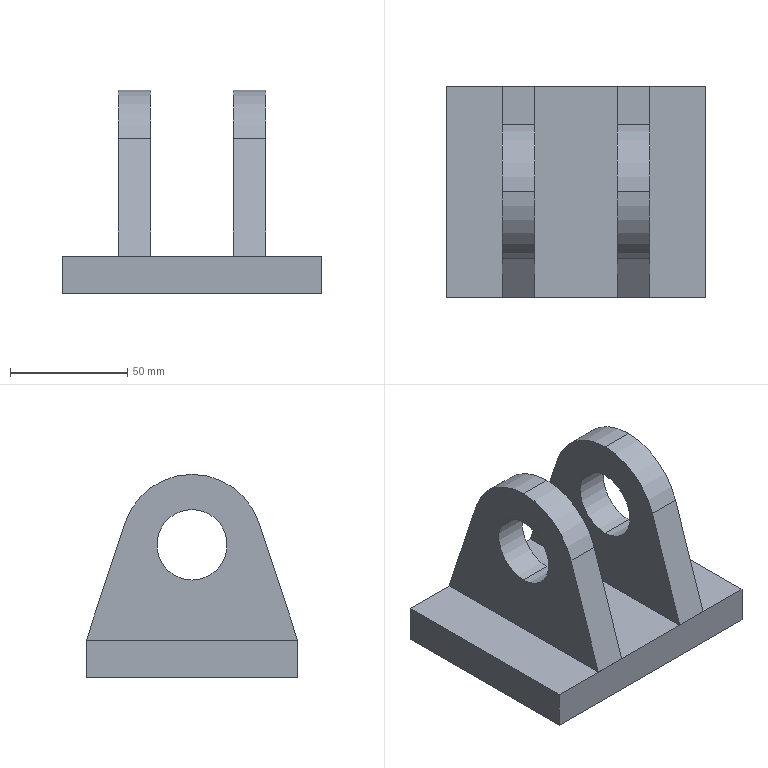Part | SolidWorks | features ICE 2, Extrusion 1, MirrorSolid 1 | 3 solids | 24 faces | box 110 x 90 x 86.592 mm | volume 265530 mm3 | plane 16 | cylinder 8 | commonest cylinder face diameters 30 x4 60 x4
STEP:
#1=CARTESIAN_POINT('',(55.,-45.,0.));
#2=VERTEX_POINT('',#1);
#3=CARTESIAN_POINT('',(55.,45.,0.));
#4=VERTEX_POINT('',#3);
#5=CARTESIAN_POINT('',(55.,-45.,0.));
#6=DIRECTION('',(0.,1.,0.));
#7=VECTOR('',#6,1000.);
#8=LINE('',#5,#7);
#9=EDGE_CURVE('',#2,#4,#8,.T.);
#10=ORIENTED_EDGE('',*,*,#9,.T.);
#11=CARTESIAN_POINT('',(55.,45.,16.));
#12=VERTEX_POINT('',#11);
#13=CARTESIAN_POINT('',(55.,45.,16.));
#14=DIRECTION('',(0.,0.,-1.));
#15=VECTOR('',#14,1000.);
#16=LINE('',#13,#15);
#17=EDGE_CURVE('',#12,#4,#16,.T.);
#18=ORIENTED_EDGE('',*,*,#17,.F.);
#19=CARTESIAN_POINT('',(55.,-45.,16.));
#20=VERTEX_POINT('',#19);
#21=CARTESIAN_POINT('',(55.,-45.,16.));
#22=DIRECTION('',(0.,1.,0.));
#23=VECTOR('',#22,1000.);
#24=LINE('',#21,#23);
#25=EDGE_CURVE('',#20,#12,#24,.T.);
#26=ORIENTED_EDGE('',*,*,#25,.F.);
#27=CARTESIAN_POINT('',(55.,-45.,16.));
#28=DIRECTION('',(0.,0.,-1.));
#29=VECTOR('',#28,1000.);
#30=LINE('',#27,#29);
#31=EDGE_CURVE('',#20,#2,#30,.T.);
#32=ORIENTED_EDGE('',*,*,#31,.T.);
#33=EDGE_LOOP('',(#10,#18,#26,#32));
#34=FACE_OUTER_BOUND('',#33,.T.);
#35=CARTESIAN_POINT('',(55.,-45.,16.));
#36=DIRECTION('',(-1.,0.,0.));
#37=DIRECTION('',(0.,0.,1.));
#38=AXIS2_PLACEMENT_3D('',#35,#36,#37);
#39=PLANE('',#38);
#40=ADVANCED_FACE('',(#34),#39,.F.);
#41=CARTESIAN_POINT('',(-55.,45.,0.));
#42=VERTEX_POINT('',#41);
#43=CARTESIAN_POINT('',(-55.,45.,0.));
#44=DIRECTION('',(-1.,0.,0.));
#45=VECTOR('',#44,1000.);
#46=LINE('',#43,#45);
#47=EDGE_CURVE('',#4,#42,#46,.T.);
#48=ORIENTED_EDGE('',*,*,#47,.T.);
#49=CARTESIAN_POINT('',(-55.,45.,16.));
#50=VERTEX_POINT('',#49);
#51=CARTESIAN_POINT('',(-55.,45.,16.));
#52=DIRECTION('',(0.,0.,-1.));
#53=VECTOR('',#52,1000.);
#54=LINE('',#51,#53);
#55=EDGE_CURVE('',#50,#42,#54,.T.);
#56=ORIENTED_EDGE('',*,*,#55,.F.);
#57=CARTESIAN_POINT('',(-55.,45.,16.));
#58=DIRECTION('',(-1.,0.,0.));
#59=VECTOR('',#58,1000.);
#60=LINE('',#57,#59);
#61=EDGE_CURVE('',#12,#50,#60,.T.);
#62=ORIENTED_EDGE('',*,*,#61,.F.);
#63=ORIENTED_EDGE('',*,*,#17,.T.);
#64=EDGE_LOOP('',(#48,#56,#62,#63));
#65=FACE_OUTER_BOUND('',#64,.T.);
#66=CARTESIAN_POINT('',(-55.,45.,16.));
#67=DIRECTION('',(0.,-1.,0.));
#68=DIRECTION('',(1.,0.,0.));
#69=AXIS2_PLACEMENT_3D('',#66,#67,#68);
#70=PLANE('',#69);
#71=ADVANCED_FACE('',(#65),#70,.F.);
#72=CARTESIAN_POINT('',(-55.,-45.,0.));
#73=VERTEX_POINT('',#72);
#74=CARTESIAN_POINT('',(-55.,-45.,0.));
#75=DIRECTION('',(0.,-1.,0.));
#76=VECTOR('',#75,1000.);
#77=LINE('',#74,#76);
#78=EDGE_CURVE('',#42,#73,#77,.T.);
#79=ORIENTED_EDGE('',*,*,#78,.T.);
#80=CARTESIAN_POINT('',(-55.,-45.,16.));
#81=VERTEX_POINT('',#80);
#82=CARTESIAN_POINT('',(-55.,-45.,16.));
#83=DIRECTION('',(0.,0.,-1.));
#84=VECTOR('',#83,1000.);
#85=LINE('',#82,#84);
#86=EDGE_CURVE('',#81,#73,#85,.T.);
#87=ORIENTED_EDGE('',*,*,#86,.F.);
#88=CARTESIAN_POINT('',(-55.,-45.,16.));
#89=DIRECTION('',(0.,-1.,0.));
#90=VECTOR('',#89,1000.);
#91=LINE('',#88,#90);
#92=EDGE_CURVE('',#50,#81,#91,.T.);
#93=ORIENTED_EDGE('',*,*,#92,.F.);
#94=ORIENTED_EDGE('',*,*,#55,.T.);
#95=EDGE_LOOP('',(#79,#87,#93,#94));
#96=FACE_OUTER_BOUND('',#95,.T.);
#97=CARTESIAN_POINT('',(-55.,-45.,16.));
#98=DIRECTION('',(1.,0.,0.));
#99=DIRECTION('',(0.,0.,-1.));
#100=AXIS2_PLACEMENT_3D('',#97,#98,#99);
#101=PLANE('',#100);
#102=ADVANCED_FACE('',(#96),#101,.F.);
#103=CARTESIAN_POINT('',(-55.,-45.,0.));
#104=DIRECTION('',(1.,0.,0.));
#105=VECTOR('',#104,1000.);
#106=LINE('',#103,#105);
#107=EDGE_CURVE('',#73,#2,#106,.T.);
#108=ORIENTED_EDGE('',*,*,#107,.T.);
#109=ORIENTED_EDGE('',*,*,#31,.F.);
#110=CARTESIAN_POINT('',(-55.,-45.,16.));
#111=DIRECTION('',(1.,0.,0.));
#112=VECTOR('',#111,1000.);
#113=LINE('',#110,#112);
#114=EDGE_CURVE('',#81,#20,#113,.T.);
#115=ORIENTED_EDGE('',*,*,#114,.F.);
#116=ORIENTED_EDGE('',*,*,#86,.T.);
#117=EDGE_LOOP('',(#108,#109,#115,#116));
#118=FACE_OUTER_BOUND('',#117,.T.);
#119=CARTESIAN_POINT('',(-55.,-45.,16.));
#120=DIRECTION('',(0.,1.,0.));
#121=DIRECTION('',(-1.,0.,0.));
#122=AXIS2_PLACEMENT_3D('',#119,#120,#121);
#123=PLANE('',#122);
#124=ADVANCED_FACE('',(#118),#123,.F.);
#125=ORIENTED_EDGE('',*,*,#25,.T.);
#126=ORIENTED_EDGE('',*,*,#61,.T.);
#127=ORIENTED_EDGE('',*,*,#92,.T.);
#128=ORIENTED_EDGE('',*,*,#114,.T.);
#129=EDGE_LOOP('',(#125,#126,#127,#128));
#130=FACE_OUTER_BOUND('',#129,.T.);
#131=CARTESIAN_POINT('',(0.,0.,16.));
#132=DIRECTION('',(0.,0.,-1.));
#133=DIRECTION('',(-1.,0.,0.));
#134=AXIS2_PLACEMENT_3D('',#131,#132,#133);
#135=PLANE('',#134);
#136=ADVANCED_FACE('',(#130),#135,.F.);
#137=ORIENTED_EDGE('',*,*,#9,.F.);
#138=ORIENTED_EDGE('',*,*,#107,.F.);
#139=ORIENTED_EDGE('',*,*,#78,.F.);
#140=ORIENTED_EDGE('',*,*,#47,.F.);
#141=EDGE_LOOP('',(#137,#138,#139,#140));
#142=FACE_OUTER_BOUND('',#141,.T.);
#143=CARTESIAN_POINT('',(0.,0.,0.));
#144=DIRECTION('',(0.,0.,-1.));
#145=DIRECTION('',(-1.,0.,0.));
#146=AXIS2_PLACEMENT_3D('',#143,#144,#145);
#147=PLANE('',#146);
#148=ADVANCED_FACE('',(#142),#147,.T.);
#149=CLOSED_SHELL('',(#40,#71,#102,#124,#136,#148));
#150=MANIFOLD_SOLID_BREP('',#149);
#151=CARTESIAN_POINT('',(17.5,0.,71.592));
#152=VERTEX_POINT('',#151);
#153=CARTESIAN_POINT('',(17.5,0.,41.592));
#154=VERTEX_POINT('',#153);
#155=CARTESIAN_POINT('',(17.5,0.,56.592));
#156=DIRECTION('',(1.,0.,0.));
#157=DIRECTION('',(0.,0.,1.));
#158=AXIS2_PLACEMENT_3D('',#155,#156,#157);
#159=CIRCLE('',#158,15.);
#160=EDGE_CURVE('',#152,#154,#159,.T.);
#161=ORIENTED_EDGE('',*,*,#160,.F.);
#162=CARTESIAN_POINT('',(31.5,0.,71.592));
#163=VERTEX_POINT('',#162);
#164=CARTESIAN_POINT('',(-55.001,0.,71.592));
#165=DIRECTION('',(1.,0.,0.));
#166=VECTOR('',#165,1000.);
#167=LINE('',#164,#166);
#168=EDGE_CURVE('',#152,#163,#167,.T.);
#169=ORIENTED_EDGE('',*,*,#168,.T.);
#170=CARTESIAN_POINT('',(31.5,0.,41.592));
#171=VERTEX_POINT('',#170);
#172=CARTESIAN_POINT('',(31.5,0.,56.592));
#173=DIRECTION('',(1.,0.,0.));
#174=DIRECTION('',(0.,0.,-1.));
#175=AXIS2_PLACEMENT_3D('',#172,#173,#174);
#176=CIRCLE('',#175,15.);
#177=EDGE_CURVE('',#163,#171,#176,.T.);
#178=ORIENTED_EDGE('',*,*,#177,.T.);
#179=CARTESIAN_POINT('',(-55.001,0.,41.592));
#180=DIRECTION('',(1.,0.,0.));
#181=VECTOR('',#180,1000.);
#182=LINE('',#179,#181);
#183=EDGE_CURVE('',#154,#171,#182,.T.);
#184=ORIENTED_EDGE('',*,*,#183,.F.);
#185=EDGE_LOOP('',(#161,#169,#178,#184));
#186=FACE_OUTER_BOUND('',#185,.T.);
#187=CARTESIAN_POINT('',(-55.001,0.,56.592));
#188=DIRECTION('',(1.,0.,0.));
#189=DIRECTION('',(0.,0.,-1.));
#190=AXIS2_PLACEMENT_3D('',#187,#188,#189);
#191=CYLINDRICAL_SURFACE('',#190,15.);
#192=ADVANCED_FACE('',(#186),#191,.F.);
#193=CARTESIAN_POINT('',(31.5,0.,86.592));
#194=VERTEX_POINT('',#193);
#195=CARTESIAN_POINT('',(31.5,-28.487,66.));
#196=VERTEX_POINT('',#195);
#197=CARTESIAN_POINT('',(31.5,0.,56.592));
#198=DIRECTION('',(1.,0.,0.));
#199=DIRECTION('',(0.,0.,1.));
#200=AXIS2_PLACEMENT_3D('',#197,#198,#199);
#201=CIRCLE('',#200,30.);
#202=EDGE_CURVE('',#194,#196,#201,.T.);
#203=ORIENTED_EDGE('',*,*,#202,.F.);
#204=CARTESIAN_POINT('',(17.5,0.,86.592));
#205=VERTEX_POINT('',#204);
#206=CARTESIAN_POINT('',(31.5,0.,86.592));
#207=DIRECTION('',(-1.,0.,0.));
#208=VECTOR('',#207,1000.);
#209=LINE('',#206,#208);
#210=EDGE_CURVE('',#194,#205,#209,.T.);
#211=ORIENTED_EDGE('',*,*,#210,.T.);
#212=CARTESIAN_POINT('',(17.5,-28.487,66.));
#213=VERTEX_POINT('',#212);
#214=CARTESIAN_POINT('',(17.5,0.,56.592));
#215=DIRECTION('',(1.,0.,0.));
#216=DIRECTION('',(0.,0.,1.));
#217=AXIS2_PLACEMENT_3D('',#214,#215,#216);
#218=CIRCLE('',#217,30.);
#219=EDGE_CURVE('',#205,#213,#218,.T.);
#220=ORIENTED_EDGE('',*,*,#219,.T.);
#221=CARTESIAN_POINT('',(31.5,-28.487,66.));
#222=DIRECTION('',(-1.,0.,0.));
#223=VECTOR('',#222,1000.);
#224=LINE('',#221,#223);
#225=EDGE_CURVE('',#196,#213,#224,.T.);
#226=ORIENTED_EDGE('',*,*,#225,.F.);
#227=EDGE_LOOP('',(#203,#211,#220,#226));
#228=FACE_OUTER_BOUND('',#227,.T.);
#229=CARTESIAN_POINT('',(31.5,0.,56.592));
#230=DIRECTION('',(-1.,0.,0.));
#231=DIRECTION('',(0.,0.,1.));
#232=AXIS2_PLACEMENT_3D('',#229,#230,#231);
#233=CYLINDRICAL_SURFACE('',#232,30.);
#234=ADVANCED_FACE('',(#228),#233,.T.);
#235=CARTESIAN_POINT('',(17.5,-45.,16.));
#236=VERTEX_POINT('',#235);
#237=CARTESIAN_POINT('',(17.5,45.,16.));
#238=VERTEX_POINT('',#237);
#239=CARTESIAN_POINT('',(17.5,45.,16.));
#240=DIRECTION('',(0.,1.,0.));
#241=VECTOR('',#240,1000.);
#242=LINE('',#239,#241);
#243=EDGE_CURVE('',#236,#238,#242,.T.);
#244=ORIENTED_EDGE('',*,*,#243,.T.);
#245=CARTESIAN_POINT('',(31.5,45.,16.));
#246=VERTEX_POINT('',#245);
#247=CARTESIAN_POINT('',(31.5,45.,16.));
#248=DIRECTION('',(-1.,0.,0.));
#249=VECTOR('',#248,1000.);
#250=LINE('',#247,#249);
#251=EDGE_CURVE('',#246,#238,#250,.T.);
#252=ORIENTED_EDGE('',*,*,#251,.F.);
#253=CARTESIAN_POINT('',(31.5,-45.,16.));
#254=VERTEX_POINT('',#253);
#255=CARTESIAN_POINT('',(31.5,45.,16.));
#256=DIRECTION('',(0.,1.,0.));
#257=VECTOR('',#256,1000.);
#258=LINE('',#255,#257);
#259=EDGE_CURVE('',#254,#246,#258,.T.);
#260=ORIENTED_EDGE('',*,*,#259,.F.);
#261=CARTESIAN_POINT('',(31.5,-45.,16.));
#262=DIRECTION('',(-1.,0.,0.));
#263=VECTOR('',#262,1000.);
#264=LINE('',#261,#263);
#265=EDGE_CURVE('',#254,#236,#264,.T.);
#266=ORIENTED_EDGE('',*,*,#265,.T.);
#267=EDGE_LOOP('',(#244,#252,#260,#266));
#268=FACE_OUTER_BOUND('',#267,.T.);
#269=CARTESIAN_POINT('',(31.5,45.,16.));
#270=DIRECTION('',(0.,0.,1.));
#271=DIRECTION('',(1.,0.,0.));
#272=AXIS2_PLACEMENT_3D('',#269,#270,#271);
#273=PLANE('',#272);
#274=ADVANCED_FACE('',(#268),#273,.F.);
#275=CARTESIAN_POINT('',(17.5,28.487,66.));
#276=VERTEX_POINT('',#275);
#277=CARTESIAN_POINT('',(17.5,45.,16.));
#278=DIRECTION('',(0.,-0.3136,0.9496));
#279=VECTOR('',#278,1000.);
#280=LINE('',#277,#279);
#281=EDGE_CURVE('',#238,#276,#280,.T.);
#282=ORIENTED_EDGE('',*,*,#281,.T.);
#283=CARTESIAN_POINT('',(31.5,28.487,66.));
#284=VERTEX_POINT('',#283);
#285=CARTESIAN_POINT('',(31.5,28.487,66.));
#286=DIRECTION('',(-1.,0.,0.));
#287=VECTOR('',#286,1000.);
#288=LINE('',#285,#287);
#289=EDGE_CURVE('',#284,#276,#288,.T.);
#290=ORIENTED_EDGE('',*,*,#289,.F.);
#291=CARTESIAN_POINT('',(31.5,45.,16.));
#292=DIRECTION('',(0.,-0.3136,0.9496));
#293=VECTOR('',#292,1000.);
#294=LINE('',#291,#293);
#295=EDGE_CURVE('',#246,#284,#294,.T.);
#296=ORIENTED_EDGE('',*,*,#295,.F.);
#297=ORIENTED_EDGE('',*,*,#251,.T.);
#298=EDGE_LOOP('',(#282,#290,#296,#297));
#299=FACE_OUTER_BOUND('',#298,.T.);
#300=CARTESIAN_POINT('',(31.5,45.,16.));
#301=DIRECTION('',(0.,-0.9496,-0.3136));
#302=DIRECTION('',(0.,0.3136,-0.9496));
#303=AXIS2_PLACEMENT_3D('',#300,#301,#302);
#304=PLANE('',#303);
#305=ADVANCED_FACE('',(#299),#304,.F.);
#306=ORIENTED_EDGE('',*,*,#210,.F.);
#307=CARTESIAN_POINT('',(31.5,0.,56.592));
#308=DIRECTION('',(1.,0.,0.));
#309=DIRECTION('',(0.,0.,1.));
#310=AXIS2_PLACEMENT_3D('',#307,#308,#309);
#311=CIRCLE('',#310,30.);
#312=EDGE_CURVE('',#284,#194,#311,.T.);
#313=ORIENTED_EDGE('',*,*,#312,.F.);
#314=ORIENTED_EDGE('',*,*,#289,.T.);
#315=CARTESIAN_POINT('',(17.5,0.,56.592));
#316=DIRECTION('',(1.,0.,0.));
#317=DIRECTION('',(0.,0.,1.));
#318=AXIS2_PLACEMENT_3D('',#315,#316,#317);
#319=CIRCLE('',#318,30.);
#320=EDGE_CURVE('',#276,#205,#319,.T.);
#321=ORIENTED_EDGE('',*,*,#320,.T.);
#322=EDGE_LOOP('',(#306,#313,#314,#321));
#323=FACE_OUTER_BOUND('',#322,.T.);
#324=CARTESIAN_POINT('',(31.5,0.,56.592));
#325=DIRECTION('',(-1.,0.,0.));
#326=DIRECTION('',(0.,0.,1.));
#327=AXIS2_PLACEMENT_3D('',#324,#325,#326);
#328=CYLINDRICAL_SURFACE('',#327,30.);
#329=ADVANCED_FACE('',(#323),#328,.T.);
#330=CARTESIAN_POINT('',(17.5,-45.,16.));
#331=DIRECTION('',(0.,-0.3136,-0.9496));
#332=VECTOR('',#331,1000.);
#333=LINE('',#330,#332);
#334=EDGE_CURVE('',#213,#236,#333,.T.);
#335=ORIENTED_EDGE('',*,*,#334,.T.);
#336=ORIENTED_EDGE('',*,*,#265,.F.);
#337=CARTESIAN_POINT('',(31.5,-45.,16.));
#338=DIRECTION('',(0.,-0.3136,-0.9496));
#339=VECTOR('',#338,1000.);
#340=LINE('',#337,#339);
#341=EDGE_CURVE('',#196,#254,#340,.T.);
#342=ORIENTED_EDGE('',*,*,#341,.F.);
#343=ORIENTED_EDGE('',*,*,#225,.T.);
#344=EDGE_LOOP('',(#335,#336,#342,#343));
#345=FACE_OUTER_BOUND('',#344,.T.);
#346=CARTESIAN_POINT('',(31.5,-45.,16.));
#347=DIRECTION('',(0.,0.9496,-0.3136));
#348=DIRECTION('',(0.,0.3136,0.9496));
#349=AXIS2_PLACEMENT_3D('',#346,#347,#348);
#350=PLANE('',#349);
#351=ADVANCED_FACE('',(#345),#350,.F.);
#352=CARTESIAN_POINT('',(31.5,0.,56.592));
#353=DIRECTION('',(1.,0.,0.));
#354=DIRECTION('',(0.,0.,-1.));
#355=AXIS2_PLACEMENT_3D('',#352,#353,#354);
#356=CIRCLE('',#355,15.);
#357=EDGE_CURVE('',#171,#163,#356,.T.);
#358=ORIENTED_EDGE('',*,*,#357,.F.);
#359=ORIENTED_EDGE('',*,*,#177,.F.);
#360=EDGE_LOOP('',(#358,#359));
#361=FACE_BOUND('',#360,.T.);
#362=ORIENTED_EDGE('',*,*,#259,.T.);
#363=ORIENTED_EDGE('',*,*,#295,.T.);
#364=ORIENTED_EDGE('',*,*,#312,.T.);
#365=ORIENTED_EDGE('',*,*,#202,.T.);
#366=ORIENTED_EDGE('',*,*,#341,.T.);
#367=EDGE_LOOP('',(#362,#363,#364,#365,#366));
#368=FACE_OUTER_BOUND('',#367,.T.);
#369=CARTESIAN_POINT('',(31.5,0.,56.592));
#370=DIRECTION('',(-1.,0.,0.));
#371=DIRECTION('',(0.,0.,1.));
#372=AXIS2_PLACEMENT_3D('',#369,#370,#371);
#373=PLANE('',#372);
#374=ADVANCED_FACE('',(#361,#368),#373,.F.);
#375=CARTESIAN_POINT('',(17.5,0.,56.592));
#376=DIRECTION('',(1.,0.,0.));
#377=DIRECTION('',(0.,0.,1.));
#378=AXIS2_PLACEMENT_3D('',#375,#376,#377);
#379=CIRCLE('',#378,15.);
#380=EDGE_CURVE('',#154,#152,#379,.T.);
#381=ORIENTED_EDGE('',*,*,#380,.T.);
#382=ORIENTED_EDGE('',*,*,#160,.T.);
#383=EDGE_LOOP('',(#381,#382));
#384=FACE_BOUND('',#383,.T.);
#385=ORIENTED_EDGE('',*,*,#243,.F.);
#386=ORIENTED_EDGE('',*,*,#334,.F.);
#387=ORIENTED_EDGE('',*,*,#219,.F.);
#388=ORIENTED_EDGE('',*,*,#320,.F.);
#389=ORIENTED_EDGE('',*,*,#281,.F.);
#390=EDGE_LOOP('',(#385,#386,#387,#388,#389));
#391=FACE_OUTER_BOUND('',#390,.T.);
#392=CARTESIAN_POINT('',(17.5,0.,56.592));
#393=DIRECTION('',(-1.,0.,0.));
#394=DIRECTION('',(0.,0.,1.));
#395=AXIS2_PLACEMENT_3D('',#392,#393,#394);
#396=PLANE('',#395);
#397=ADVANCED_FACE('',(#384,#391),#396,.T.);
#398=ORIENTED_EDGE('',*,*,#168,.F.);
#399=ORIENTED_EDGE('',*,*,#380,.F.);
#400=ORIENTED_EDGE('',*,*,#183,.T.);
#401=ORIENTED_EDGE('',*,*,#357,.T.);
#402=EDGE_LOOP('',(#398,#399,#400,#401));
#403=FACE_OUTER_BOUND('',#402,.T.);
#404=CARTESIAN_POINT('',(-55.001,0.,56.592));
#405=DIRECTION('',(1.,0.,0.));
#406=DIRECTION('',(0.,0.,-1.));
#407=AXIS2_PLACEMENT_3D('',#404,#405,#406);
#408=CYLINDRICAL_SURFACE('',#407,15.);
#409=ADVANCED_FACE('',(#403),#408,.F.);
#410=CLOSED_SHELL('',(#192,#234,#274,#305,#329,#351,#374,#397,#409));
#411=MANIFOLD_SOLID_BREP('',#410);
#412=CARTESIAN_POINT('',(-17.5,0.,41.592));
#413=VERTEX_POINT('',#412);
#414=CARTESIAN_POINT('',(-17.5,0.,71.592));
#415=VERTEX_POINT('',#414);
#416=CARTESIAN_POINT('',(-17.5,0.,56.592));
#417=DIRECTION('',(1.,0.,0.));
#418=DIRECTION('',(0.,0.,1.));
#419=AXIS2_PLACEMENT_3D('',#416,#417,#418);
#420=CIRCLE('',#419,15.);
#421=EDGE_CURVE('',#413,#415,#420,.T.);
#422=ORIENTED_EDGE('',*,*,#421,.T.);
#423=CARTESIAN_POINT('',(-31.5,0.,71.592));
#424=VERTEX_POINT('',#423);
#425=CARTESIAN_POINT('',(55.001,0.,71.592));
#426=DIRECTION('',(-1.,0.,0.));
#427=VECTOR('',#426,1000.);
#428=LINE('',#425,#427);
#429=EDGE_CURVE('',#415,#424,#428,.T.);
#430=ORIENTED_EDGE('',*,*,#429,.T.);
#431=CARTESIAN_POINT('',(-31.5,0.,41.592));
#432=VERTEX_POINT('',#431);
#433=CARTESIAN_POINT('',(-31.5,0.,56.592));
#434=DIRECTION('',(1.,0.,0.));
#435=DIRECTION('',(0.,0.,-1.));
#436=AXIS2_PLACEMENT_3D('',#433,#434,#435);
#437=CIRCLE('',#436,15.);
#438=EDGE_CURVE('',#432,#424,#437,.T.);
#439=ORIENTED_EDGE('',*,*,#438,.F.);
#440=CARTESIAN_POINT('',(55.001,0.,41.592));
#441=DIRECTION('',(-1.,0.,0.));
#442=VECTOR('',#441,1000.);
#443=LINE('',#440,#442);
#444=EDGE_CURVE('',#413,#432,#443,.T.);
#445=ORIENTED_EDGE('',*,*,#444,.F.);
#446=EDGE_LOOP('',(#422,#430,#439,#445));
#447=FACE_OUTER_BOUND('',#446,.T.);
#448=CARTESIAN_POINT('',(55.001,0.,56.592));
#449=DIRECTION('',(-1.,0.,0.));
#450=DIRECTION('',(0.,0.,-1.));
#451=AXIS2_PLACEMENT_3D('',#448,#449,#450);
#452=CYLINDRICAL_SURFACE('',#451,15.);
#453=ADVANCED_FACE('',(#447),#452,.F.);
#454=CARTESIAN_POINT('',(-31.5,28.487,66.));
#455=VERTEX_POINT('',#454);
#456=CARTESIAN_POINT('',(-31.5,0.,86.592));
#457=VERTEX_POINT('',#456);
#458=CARTESIAN_POINT('',(-31.5,0.,56.592));
#459=DIRECTION('',(1.,0.,0.));
#460=DIRECTION('',(0.,0.,1.));
#461=AXIS2_PLACEMENT_3D('',#458,#459,#460);
#462=CIRCLE('',#461,30.);
#463=EDGE_CURVE('',#455,#457,#462,.T.);
#464=ORIENTED_EDGE('',*,*,#463,.T.);
#465=CARTESIAN_POINT('',(-17.5,0.,86.592));
#466=VERTEX_POINT('',#465);
#467=CARTESIAN_POINT('',(-31.5,0.,86.592));
#468=DIRECTION('',(1.,0.,0.));
#469=VECTOR('',#468,1000.);
#470=LINE('',#467,#469);
#471=EDGE_CURVE('',#457,#466,#470,.T.);
#472=ORIENTED_EDGE('',*,*,#471,.T.);
#473=CARTESIAN_POINT('',(-17.5,28.487,66.));
#474=VERTEX_POINT('',#473);
#475=CARTESIAN_POINT('',(-17.5,0.,56.592));
#476=DIRECTION('',(1.,0.,0.));
#477=DIRECTION('',(0.,0.,1.));
#478=AXIS2_PLACEMENT_3D('',#475,#476,#477);
#479=CIRCLE('',#478,30.);
#480=EDGE_CURVE('',#474,#466,#479,.T.);
#481=ORIENTED_EDGE('',*,*,#480,.F.);
#482=CARTESIAN_POINT('',(-31.5,28.487,66.));
#483=DIRECTION('',(1.,0.,0.));
#484=VECTOR('',#483,1000.);
#485=LINE('',#482,#484);
#486=EDGE_CURVE('',#455,#474,#485,.T.);
#487=ORIENTED_EDGE('',*,*,#486,.F.);
#488=EDGE_LOOP('',(#464,#472,#481,#487));
#489=FACE_OUTER_BOUND('',#488,.T.);
#490=CARTESIAN_POINT('',(-31.5,0.,56.592));
#491=DIRECTION('',(1.,0.,0.));
#492=DIRECTION('',(0.,0.,1.));
#493=AXIS2_PLACEMENT_3D('',#490,#491,#492);
#494=CYLINDRICAL_SURFACE('',#493,30.);
#495=ADVANCED_FACE('',(#489),#494,.T.);
#496=CARTESIAN_POINT('',(-17.5,-45.,16.));
#497=VERTEX_POINT('',#496);
#498=CARTESIAN_POINT('',(-17.5,45.,16.));
#499=VERTEX_POINT('',#498);
#500=CARTESIAN_POINT('',(-17.5,45.,16.));
#501=DIRECTION('',(0.,1.,0.));
#502=VECTOR('',#501,1000.);
#503=LINE('',#500,#502);
#504=EDGE_CURVE('',#497,#499,#503,.T.);
#505=ORIENTED_EDGE('',*,*,#504,.F.);
#506=CARTESIAN_POINT('',(-31.5,-45.,16.));
#507=VERTEX_POINT('',#506);
#508=CARTESIAN_POINT('',(-31.5,-45.,16.));
#509=DIRECTION('',(1.,0.,0.));
#510=VECTOR('',#509,1000.);
#511=LINE('',#508,#510);
#512=EDGE_CURVE('',#507,#497,#511,.T.);
#513=ORIENTED_EDGE('',*,*,#512,.F.);
#514=CARTESIAN_POINT('',(-31.5,45.,16.));
#515=VERTEX_POINT('',#514);
#516=CARTESIAN_POINT('',(-31.5,45.,16.));
#517=DIRECTION('',(0.,1.,0.));
#518=VECTOR('',#517,1000.);
#519=LINE('',#516,#518);
#520=EDGE_CURVE('',#507,#515,#519,.T.);
#521=ORIENTED_EDGE('',*,*,#520,.T.);
#522=CARTESIAN_POINT('',(-31.5,45.,16.));
#523=DIRECTION('',(1.,0.,0.));
#524=VECTOR('',#523,1000.);
#525=LINE('',#522,#524);
#526=EDGE_CURVE('',#515,#499,#525,.T.);
#527=ORIENTED_EDGE('',*,*,#526,.T.);
#528=EDGE_LOOP('',(#505,#513,#521,#527));
#529=FACE_OUTER_BOUND('',#528,.T.);
#530=CARTESIAN_POINT('',(-31.5,45.,16.));
#531=DIRECTION('',(0.,0.,1.));
#532=DIRECTION('',(-1.,0.,0.));
#533=AXIS2_PLACEMENT_3D('',#530,#531,#532);
#534=PLANE('',#533);
#535=ADVANCED_FACE('',(#529),#534,.F.);
#536=CARTESIAN_POINT('',(-17.5,45.,16.));
#537=DIRECTION('',(0.,-0.3136,0.9496));
#538=VECTOR('',#537,1000.);
#539=LINE('',#536,#538);
#540=EDGE_CURVE('',#499,#474,#539,.T.);
#541=ORIENTED_EDGE('',*,*,#540,.F.);
#542=ORIENTED_EDGE('',*,*,#526,.F.);
#543=CARTESIAN_POINT('',(-31.5,45.,16.));
#544=DIRECTION('',(0.,-0.3136,0.9496));
#545=VECTOR('',#544,1000.);
#546=LINE('',#543,#545);
#547=EDGE_CURVE('',#515,#455,#546,.T.);
#548=ORIENTED_EDGE('',*,*,#547,.T.);
#549=ORIENTED_EDGE('',*,*,#486,.T.);
#550=EDGE_LOOP('',(#541,#542,#548,#549));
#551=FACE_OUTER_BOUND('',#550,.T.);
#552=CARTESIAN_POINT('',(-31.5,45.,16.));
#553=DIRECTION('',(0.,-0.9496,-0.3136));
#554=DIRECTION('',(0.,0.3136,-0.9496));
#555=AXIS2_PLACEMENT_3D('',#552,#553,#554);
#556=PLANE('',#555);
#557=ADVANCED_FACE('',(#551),#556,.F.);
#558=ORIENTED_EDGE('',*,*,#471,.F.);
#559=CARTESIAN_POINT('',(-31.5,-28.487,66.));
#560=VERTEX_POINT('',#559);
#561=CARTESIAN_POINT('',(-31.5,0.,56.592));
#562=DIRECTION('',(1.,0.,0.));
#563=DIRECTION('',(0.,0.,1.));
#564=AXIS2_PLACEMENT_3D('',#561,#562,#563);
#565=CIRCLE('',#564,30.);
#566=EDGE_CURVE('',#457,#560,#565,.T.);
#567=ORIENTED_EDGE('',*,*,#566,.T.);
#568=CARTESIAN_POINT('',(-17.5,-28.487,66.));
#569=VERTEX_POINT('',#568);
#570=CARTESIAN_POINT('',(-31.5,-28.487,66.));
#571=DIRECTION('',(1.,0.,0.));
#572=VECTOR('',#571,1000.);
#573=LINE('',#570,#572);
#574=EDGE_CURVE('',#560,#569,#573,.T.);
#575=ORIENTED_EDGE('',*,*,#574,.T.);
#576=CARTESIAN_POINT('',(-17.5,0.,56.592));
#577=DIRECTION('',(1.,0.,0.));
#578=DIRECTION('',(0.,0.,1.));
#579=AXIS2_PLACEMENT_3D('',#576,#577,#578);
#580=CIRCLE('',#579,30.);
#581=EDGE_CURVE('',#466,#569,#580,.T.);
#582=ORIENTED_EDGE('',*,*,#581,.F.);
#583=EDGE_LOOP('',(#558,#567,#575,#582));
#584=FACE_OUTER_BOUND('',#583,.T.);
#585=CARTESIAN_POINT('',(-31.5,0.,56.592));
#586=DIRECTION('',(1.,0.,0.));
#587=DIRECTION('',(0.,0.,1.));
#588=AXIS2_PLACEMENT_3D('',#585,#586,#587);
#589=CYLINDRICAL_SURFACE('',#588,30.);
#590=ADVANCED_FACE('',(#584),#589,.T.);
#591=CARTESIAN_POINT('',(-17.5,-45.,16.));
#592=DIRECTION('',(0.,-0.3136,-0.9496));
#593=VECTOR('',#592,1000.);
#594=LINE('',#591,#593);
#595=EDGE_CURVE('',#569,#497,#594,.T.);
#596=ORIENTED_EDGE('',*,*,#595,.F.);
#597=ORIENTED_EDGE('',*,*,#574,.F.);
#598=CARTESIAN_POINT('',(-31.5,-45.,16.));
#599=DIRECTION('',(0.,-0.3136,-0.9496));
#600=VECTOR('',#599,1000.);
#601=LINE('',#598,#600);
#602=EDGE_CURVE('',#560,#507,#601,.T.);
#603=ORIENTED_EDGE('',*,*,#602,.T.);
#604=ORIENTED_EDGE('',*,*,#512,.T.);
#605=EDGE_LOOP('',(#596,#597,#603,#604));
#606=FACE_OUTER_BOUND('',#605,.T.);
#607=CARTESIAN_POINT('',(-31.5,-45.,16.));
#608=DIRECTION('',(0.,0.9496,-0.3136));
#609=DIRECTION('',(0.,0.3136,0.9496));
#610=AXIS2_PLACEMENT_3D('',#607,#608,#609);
#611=PLANE('',#610);
#612=ADVANCED_FACE('',(#606),#611,.F.);
#613=ORIENTED_EDGE('',*,*,#438,.T.);
#614=CARTESIAN_POINT('',(-31.5,0.,56.592));
#615=DIRECTION('',(1.,0.,0.));
#616=DIRECTION('',(0.,0.,-1.));
#617=AXIS2_PLACEMENT_3D('',#614,#615,#616);
#618=CIRCLE('',#617,15.);
#619=EDGE_CURVE('',#424,#432,#618,.T.);
#620=ORIENTED_EDGE('',*,*,#619,.T.);
#621=EDGE_LOOP('',(#613,#620));
#622=FACE_BOUND('',#621,.T.);
#623=ORIENTED_EDGE('',*,*,#520,.F.);
#624=ORIENTED_EDGE('',*,*,#602,.F.);
#625=ORIENTED_EDGE('',*,*,#566,.F.);
#626=ORIENTED_EDGE('',*,*,#463,.F.);
#627=ORIENTED_EDGE('',*,*,#547,.F.);
#628=EDGE_LOOP('',(#623,#624,#625,#626,#627));
#629=FACE_OUTER_BOUND('',#628,.T.);
#630=CARTESIAN_POINT('',(-31.5,0.,56.592));
#631=DIRECTION('',(1.,0.,0.));
#632=DIRECTION('',(0.,0.,1.));
#633=AXIS2_PLACEMENT_3D('',#630,#631,#632);
#634=PLANE('',#633);
#635=ADVANCED_FACE('',(#622,#629),#634,.F.);
#636=ORIENTED_EDGE('',*,*,#421,.F.);
#637=CARTESIAN_POINT('',(-17.5,0.,56.592));
#638=DIRECTION('',(1.,0.,0.));
#639=DIRECTION('',(0.,0.,1.));
#640=AXIS2_PLACEMENT_3D('',#637,#638,#639);
#641=CIRCLE('',#640,15.);
#642=EDGE_CURVE('',#415,#413,#641,.T.);
#643=ORIENTED_EDGE('',*,*,#642,.F.);
#644=EDGE_LOOP('',(#636,#643));
#645=FACE_BOUND('',#644,.T.);
#646=ORIENTED_EDGE('',*,*,#504,.T.);
#647=ORIENTED_EDGE('',*,*,#540,.T.);
#648=ORIENTED_EDGE('',*,*,#480,.T.);
#649=ORIENTED_EDGE('',*,*,#581,.T.);
#650=ORIENTED_EDGE('',*,*,#595,.T.);
#651=EDGE_LOOP('',(#646,#647,#648,#649,#650));
#652=FACE_OUTER_BOUND('',#651,.T.);
#653=CARTESIAN_POINT('',(-17.5,0.,56.592));
#654=DIRECTION('',(1.,0.,0.));
#655=DIRECTION('',(0.,0.,1.));
#656=AXIS2_PLACEMENT_3D('',#653,#654,#655);
#657=PLANE('',#656);
#658=ADVANCED_FACE('',(#645,#652),#657,.T.);
#659=ORIENTED_EDGE('',*,*,#429,.F.);
#660=ORIENTED_EDGE('',*,*,#642,.T.);
#661=ORIENTED_EDGE('',*,*,#444,.T.);
#662=ORIENTED_EDGE('',*,*,#619,.F.);
#663=EDGE_LOOP('',(#659,#660,#661,#662));
#664=FACE_OUTER_BOUND('',#663,.T.);
#665=CARTESIAN_POINT('',(55.001,0.,56.592));
#666=DIRECTION('',(-1.,0.,0.));
#667=DIRECTION('',(0.,0.,-1.));
#668=AXIS2_PLACEMENT_3D('',#665,#666,#667);
#669=CYLINDRICAL_SURFACE('',#668,15.);
#670=ADVANCED_FACE('',(#664),#669,.F.);
#671=CLOSED_SHELL('',(#453,#495,#535,#557,#590,#612,#635,#658,#670));
#672=MANIFOLD_SOLID_BREP('',#671);
#673=CARTESIAN_POINT('',(0.,0.,0.));
#674=DIRECTION('',(0.,0.,1.));
#675=DIRECTION('',(1.,0.,0.));
#676=AXIS2_PLACEMENT_3D('',#673,#674,#675);
#677=(LENGTH_UNIT()NAMED_UNIT(*)SI_UNIT(.MILLI.,.METRE.));
#678=UNCERTAINTY_MEASURE_WITH_UNIT(LENGTH_MEASURE(0.00001),#677,'','');
#679=(NAMED_UNIT(*)PLANE_ANGLE_UNIT()SI_UNIT($,.RADIAN.));
#680=(NAMED_UNIT(*)SI_UNIT($,.STERADIAN.)SOLID_ANGLE_UNIT());
#681=(GEOMETRIC_REPRESENTATION_CONTEXT(3)GLOBAL_UNCERTAINTY_ASSIGNED_CONTEXT((#678))GLOBAL_UNIT_ASSIGNED_CONTEXT((#677,#679,#680))REPRESENTATION_CONTEXT('',''));
#682=ADVANCED_BREP_SHAPE_REPRESENTATION('',(#150,#411,#672,#676),#681);